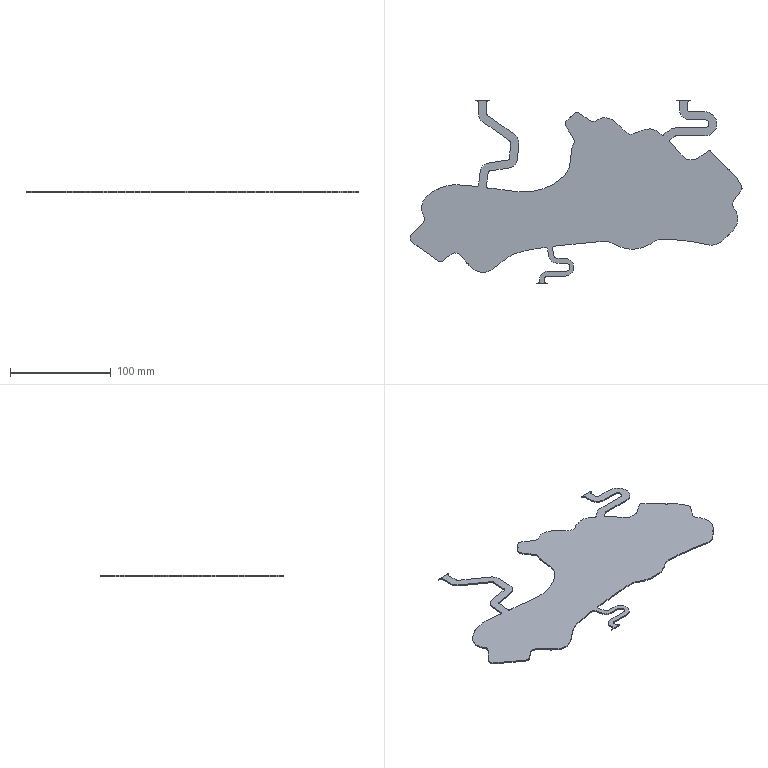Part | STEP file | gslz 2016.10.28-13_id226_x_t | 1 solid | 160 faces | box 330.211 x 182.504 x 1.25 mm | volume 36974 mm3 | cylinder 83 | plane 77 | commonest cylinder face diameters 4 x26 6 x10 20 x8 10 x7 30 x4 12 x3